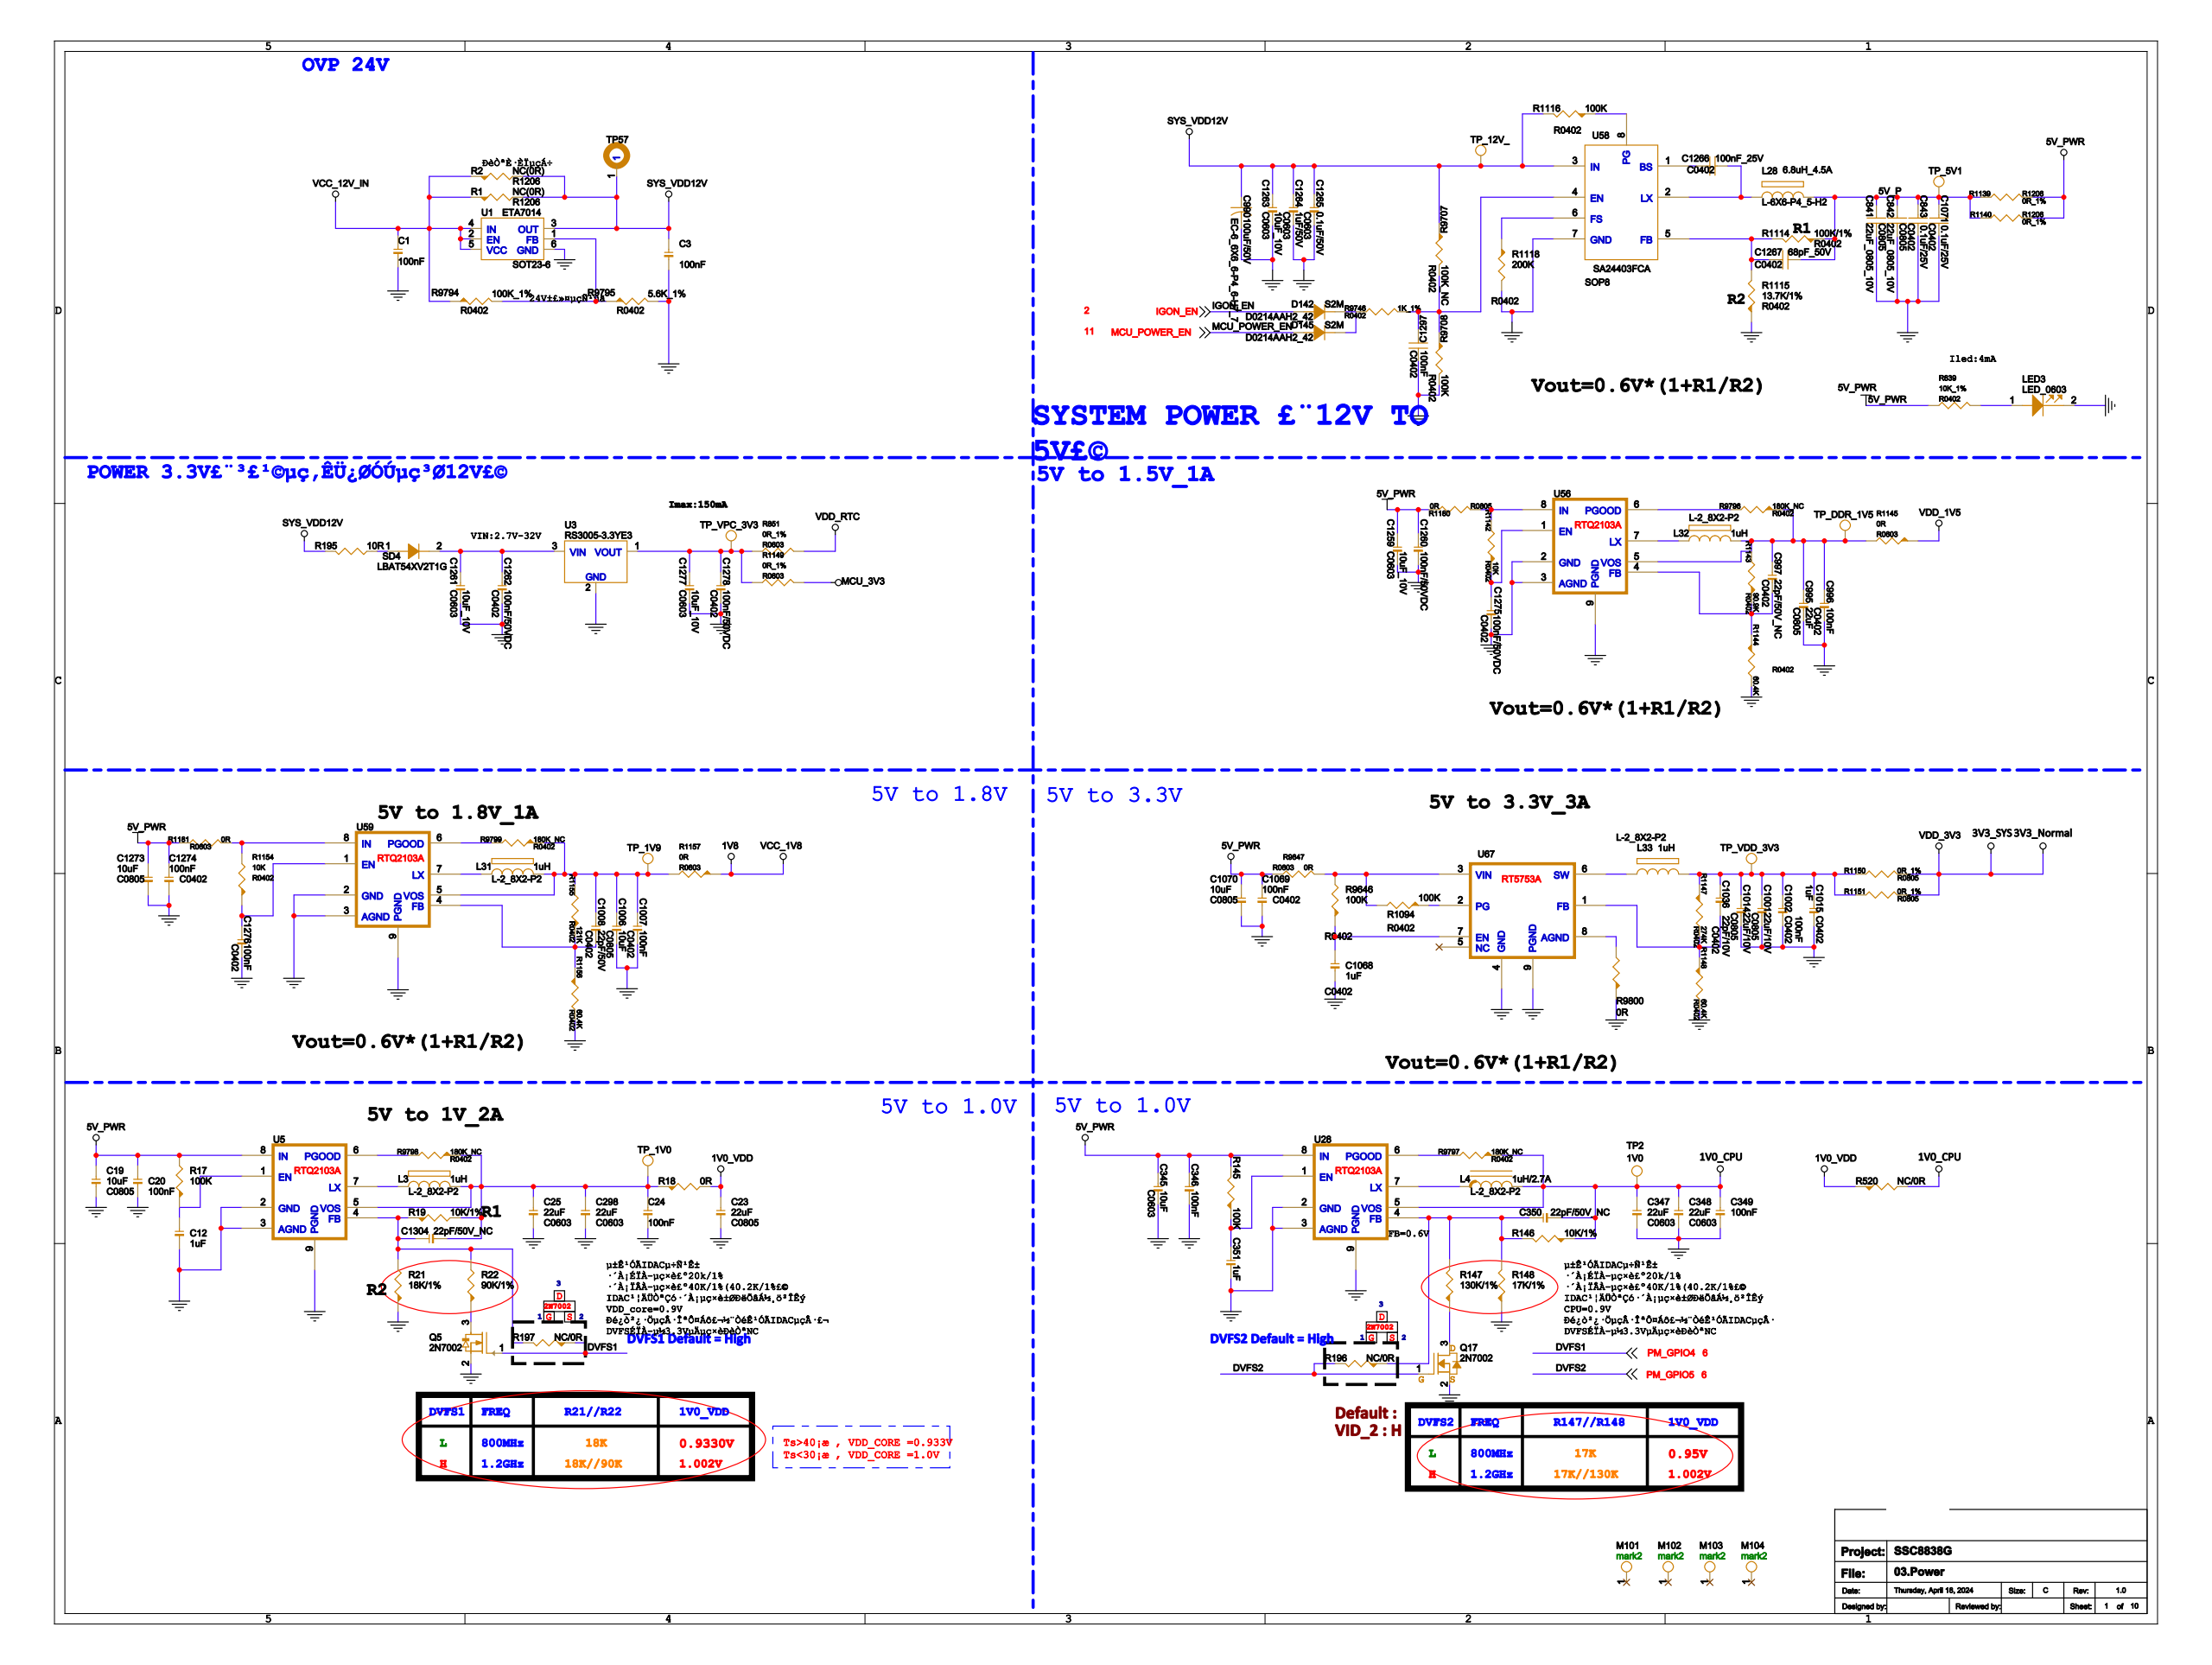Circuit board | Cadence Allegro | 958 parts | 601 nets | one sheet of the schematic
Parts on this sheet (reference | value | footprint):
C1 | 100nF | C0402
C3 | 100nF | C0402
C12 | 1uF | C0402
C19 | 10uF | C0805
C20 | 100nF | C0402
C23 | 22uF | C0805
C24 | 100nF | C0402
C25 | 22uF | C0603
C298 | 22uF | C0603
C345 | 10uF | C0603
C346 | 100nF | C0402
C347 | 22uF | C0603
C348 | 22uF | C0603
C349 | 100nF | C0402
C350 | 22pF/50V_NC | C0402
C351 | 1uF | C0402
C841 | 22uF_0805_10V | C0805
C842 | 22uF_0805_10V | C0805
C843 | 0.1uF/25V | C0402
C990 | 100uF/50V | EC-6_6X6_6-P4_6-H7_7
C995 | 22uF | C0805
C996 | 100nF | C0402
C997 | 22pF/50V_NC | C0402
C1001 | 22uF/10V | C0805
C1002 | 100nF | C0402
C1006 | 10uF | C0805
C1007 | 100nF | C0402
C1008 | 22pF/50V | C0402
C1014 | 22uF/10V | C0805
C1015 | 1uF | C0402
C1036 | 22pF/10V | C0402
C1068 | 1uF | C0402
C1069 | 100nF | C0402
C1070 | 10uF | C0805
C1071 | 0.1uF/25V | C0402
C1259 | 10uF_10V | C0603
C1260 | 100nF/50VDC | C0402
C1261 | 10uF_10V | C0603
C1262 | 100nF/50VDC | C0402
C1263 | 10uF_10V | C0603
C1264 | 1uF/50V | C0603
C1265 | 0.1uF/50V | C0603
C1266 | 100nF_25V | C0402
C1267 | 68pF_50V | C0402
C1273 | 10uF | C0805
C1274 | 100nF | C0402
C1275 | 100nF/50VDC | C0402
C1276 | 100nF | C0402
C1277 | 10uF_10V | C0603
C1278 | 100nF/50VDC | C0402
C1297 | 100nF | C0402
C1304 | 22pF/50V_NC | C0402
D142 | S2M | D0214AAH2_42
D145 | S2M | D0214AAH2_42
L3 | 1uH | L-2_8X2-P2
L4 | 1uH/2.7A | L-2_8X2-P2
L28 | 6.8uH_4.5A | L-6X6-P4_5-H2
L31 | 1uH | L-2_8X2-P2
L32 | 1uH | L-2_8X2-P2
L33 | 1uH | L-2_8X2-P2
LED3 | LED_0603 | LED-0603
Q5 | 2N7002 | SOT-23
Q17 | 2N7002 | SOT-23
R1 | NC(0R) | R1206
R2 | NC(0R) | R1206
R17 | 100K | R0402
R18 | 0R | R0603
R19 | 10K/1% | R0402
R21 | 18K/1% | R0402
R22 | 90K/1% | R0402
R145 | 100K | R0402
R146 | 10K/1% | R0402
R147 | 130K/1% | R0402
R148 | 17K/1% | R0402
R195 | 10R | R1206
R196 | NC/0R | R0402
R197 | NC/0R | R0402
R520 | NC/0R | R0603
R839 | 10K_1% | R0402
R851 | 0R_1% | R0603
R1094 | 100K | R0402
R1114 | 100K/1% | R0402
R1115 | 13.7K/1% | R0402
R1116 | 100K | R0402
R1118 | 200K | R0402
R1139 | 0R_1% | R1206
R1140 | 0R_1% | R1206
R1142 | 10K | R0402
R1143 | 90.9K | R0402
R1144 | 60.4K | R0402
R1145 | 0R | R0603
R1147 | 274K | R0402
R1148 | 60.4K | R0402
R1149 | 0R_1% | R0603
R1150 | 0R_1% | R0805
R1151 | 0R_1% | R0805
R1154 | 10K | R0402
R1155 | 121K | R0402
R1156 | 60.4K | R0402
R1157 | 0R | R0603
R1180 | 0R | R0805
R1181 | 0R | R0603
R9646 | 100K | R0402
R9647 | 0R | R0603
R9707 | 100K_NC | R0402
R9708 | 100K | R0402
R9746 | 1K_1% | R0402
R9794 | 100K_1% | R0402
R9795 | 5.6K_1% | R0402
R9796 | 180K_NC | R0402
R9797 | 180K_NC | R0402
R9798 | 180K_NC | R0402
R9799 | 180K_NC | R0402
R9800 | 0R | R0402
SD4 | LBAT54XV2T1G | SOD523
TP2 | 1V0 | TP-C40
TP57 | HOLE | TP-C40
TP_1V0 | Test_Point | TP-C40
TP_1V9 | Test_Point | TP-C40
TP_5V1 | Test_Point | TP-C40
TP_12V_ | Test_Point | TP-C40
TP_DDR_1V5 | Test_Point | TP-C40
TP_VDD_3V3 | Test_Point | TP-C40
TP_VPC_3V3 | Test_Point | TP-C40
U1 | ETA7014 | SOT23-6
U3 | RS3005-3.3YE3 | SOT-89-3
U5 | RTQ2103A | ESOP8_H
U28 | RTQ2103A | ESOP8_H
U56 | RTQ2103A | ESOP8_H
U58 | SA24403FCA | SOP8
U59 | RTQ2103A | ESOP8_H
U67 | RT5753A | DFN8-0_5-2X2X0_85T
Nets of these parts (net: part-pin ...):
VCC_12V_IN: C1-1 R1-1 R2-1 R9794-1 U1-2 U1-4 U1-5
GND: C1-2 C3-2 C12-2 C19-2 C20-2 C23-2 C24-2 C25-2 C298-2 C345-1 C346-1 C347-1 C348-1 C349-1 C351-1 C841-2 C842-2 C843-1 C990-2 C995-2 C996-2 C1001-2 C1002-2 C1006-2 C1007-2 C1014-2 C1015-2 C1068-2 C1069-2 C1070-2 C1071-1 C1259-1 C1260-1 C1261-1 C1262-1 C1263-1 C1264-1 C1265-1 C1273-2 C1274-2 C1275-2 C1276-2 C1277-1 C1278-1 C1297-1 LED3-2 Q5-2 Q17-2 R21-1 R148-1 R1115-1 R1118-2 R1144-2 R1148-2 R1156-2 R9708-2 R9795-2 R9800-1 U1-6 U3-2 U5-2 U5-3 U5-9 U28-2 U28-3 U28-9 U56-2 U56-3 U56-9 U58-7 U59-2 U59-3 U59-9 U67-4 U67-9
N21877248: C1001-1 C1002-1 C1014-1 C1015-1 C1036-1 L33-2 R1147-1 R1150-1 R1151-1 TP_VDD_3V3-1
N21855515: C1006-1 C1007-1 C1008-1 L31-2 R1155-2 R1157-2 R9799-1 TP_1V9-1 U59-5
5V_PWR: C19-1 C20-1 C345-2 C346-2 C1069-1 C1070-1 C1259-2 C1260-2 C1273-1 C1274-1 R17-2 R145-2 R839-1 R1139-2 R1140-2 R1180-1 R1181-1 R9647-1 U5-8 U28-8
N21853660: C1276-1 R1154-1 U59-1
N21851930: C24-1 C25-1 C298-1 C1304-1 L3-2 R18-1 R19-2 R9798-1 TP_1V0-1 U5-5
SYS_VDD12V: C3-1 C990-1 C1263-2 C1264-2 C1265-2 R1-2 R2-2 R195-2 R1116-2 R9707-1 TP57-1 TP_12V_-1 U1-3 U58-3
3V3_NORMAL: R1150-2 R1151-2
1V0_VDD: C23-1 R18-2 R520-1
1V0_CPU: C347-2 C348-2 C349-2 C350-1 L4-2 R146-1 R520-2 R9797-1 TP2-1 U28-5
N21840339: C995-1 C996-1 C997-1 L32-2 R1143-2 R1145-2 R9796-1 TP_DDR_1V5-1 U56-5
1V5_DRAM: R1145-1
N21877139: C1008-2 R1155-1 R1156-1 U59-4
N21877234: C1068-1 R9646-1 U67-7
N21851481: C12-1 R17-1 U5-1
N21877251: C1036-2 R1147-2 R1148-1 U67-1
5V_P: C841-1 C842-1 C843-2 C1071-2 C1267-1 L28-2 R1114-1 R1139-1 R1140-1 TP_5V1-1
VDD_RTC: R851-2
N21877365: C1297-2 R9707-2 R9708-1 R9746-2 U58-4
N21877170: C1261-2 C1262-2 SD4-2 U3-3
N21877163: C1277-2 C1278-2 R851-1 R1149-1 TP_VPC_3V3-1 U3-1
N21877318: C1266-1 L28-1 U58-2
N21877325: C1266-2 U58-1
N21877319: C1267-2 R1114-2 R1115-2 U58-5
N21840745: C1275-1 R1142-1 U56-1
N21851874: C1304-2 R19-1 R21-2 R22-2 R197-2 U5-4
N21846066: C350-2 R146-2 R147-2 R148-2 R196-1 U28-4
N21846861: C351-2 R145-1 U28-1
N21877213: C997-2 R1143-1 R1144-1 U56-4
IGON_EN: D142-1
N21877367: D142-2 D145-2 R9746-1
MCU_POWER_EN: D145-1
1V8: R1157-1
MCU_3V3: R1149-2
N21877044: L3-1 U5-7
N21877142: L31-1 U59-7
N21877201: L32-1 U56-7
N21877245: L33-1 U67-6
N21845973: L4-1 U28-7
N21877306: LED3-1 R839-2
PM_GPIO5: Q17-1 R196-2
N21877121: Q17-3 R147-1
PM_GPIO4: Q5-1 R197-1
N21877058: Q5-3 R22-1
N21971095: R1094-1 U67-2
N21877233: R1094-2 R9646-2 R9647-2 U67-3
N21877341: R1116-1 U58-8
N21877345: R1118-1 U58-6
N21877194: R1142-2 R1180-2 U56-8
N21853656: R1154-2 R1181-2 U59-8
N21877246: R9800-2 U67-8
N21877393: R195-1 SD4-1
N21877403: R9794-2 R9795-1 U1-1
N21840482: R9796-2 U56-6
N21846417: R9797-2 U28-6
N21852714: R9798-2 U5-6
N21855519: R9799-2 U59-6